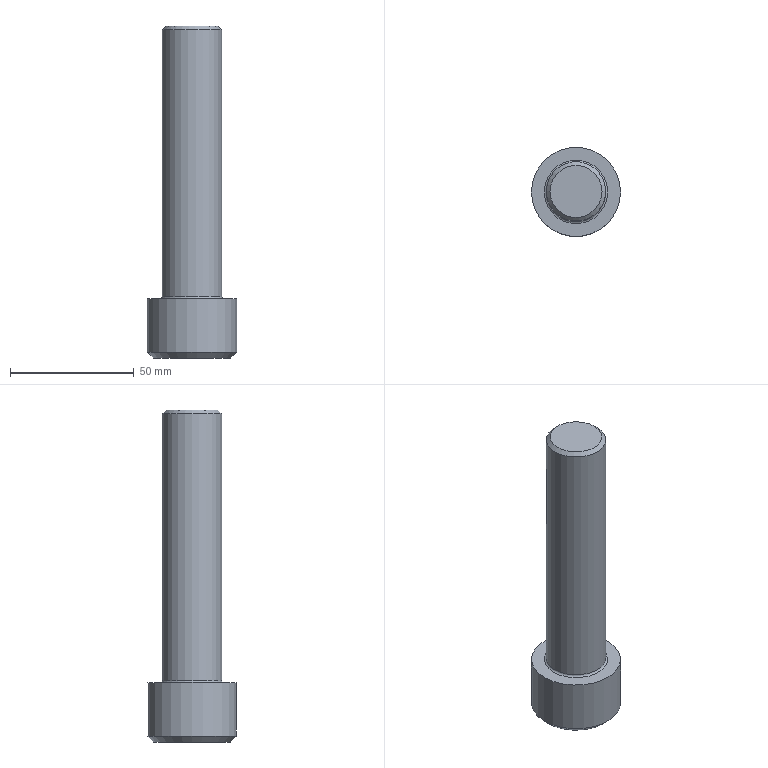Part | STEP file | solid 66 | 1 solid | 21 faces | box 36 x 36 x 134 mm | volume 70042 mm3 | plane 10 | sphere 6 | cylinder 2 | cone 2 | torus 1 | commonest cylinder face diameters 24 x1 36 x1